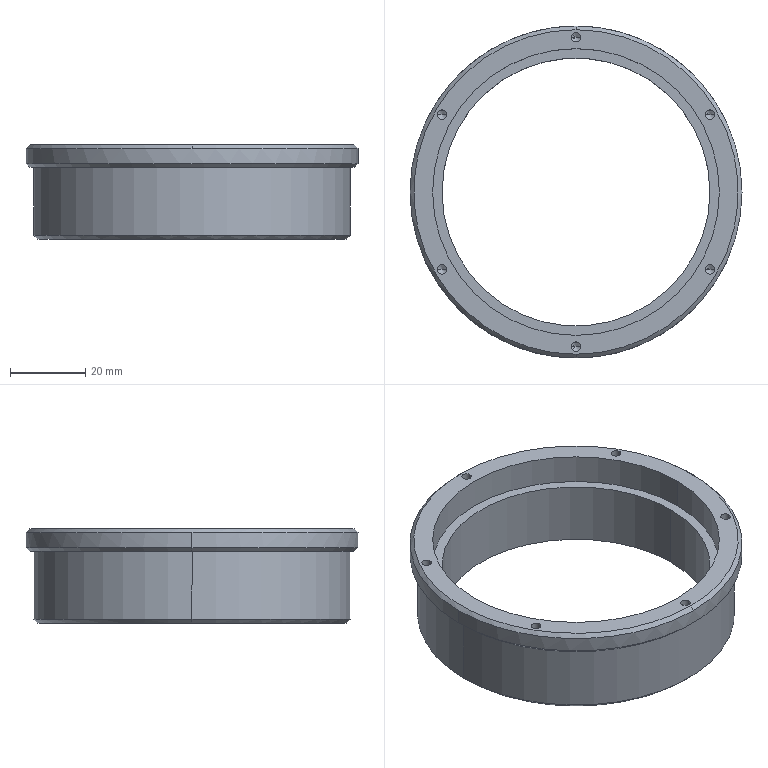Part | SolidWorks | features BaseBody 1 | 1 solid | 66 faces | box 88 x 88 x 25 mm | volume 37444 mm3 | cylinder 32 | cone 30 | plane 4 | commonest cylinder face diameters 2.5 x24 71 x2 76 x2 84 x2 88 x2